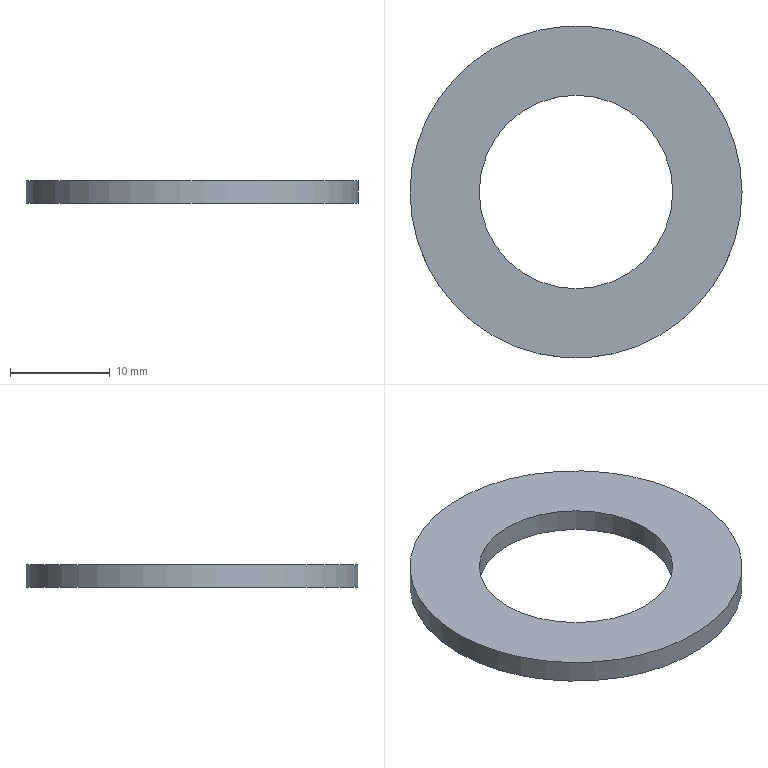Part | NX | features solid 2 | 1 solid | 4 faces | box 33.325 x 33.325 x 2.286 mm | volume 1316 mm3 | cylinder 2 | plane 2 | commonest cylinder face diameters 19.431 x1 33.325 x1
STEP:
#1=CARTESIAN_POINT('',(16.662,0.,2.286));
#2=VERTEX_POINT('',#1);
#3=CARTESIAN_POINT('',(0.,0.,2.286));
#4=DIRECTION('',(0.,0.,-1.));
#5=DIRECTION('',(1.,0.,0.));
#6=AXIS2_PLACEMENT_3D('',#3,#4,#5);
#7=CIRCLE('',#6,16.662);
#8=EDGE_CURVE('',#2,#2,#7,.T.);
#9=ORIENTED_EDGE('',*,*,#8,.T.);
#10=EDGE_LOOP('',(#9));
#11=FACE_BOUND('',#10,.T.);
#12=CARTESIAN_POINT('',(16.662,0.,0.));
#13=VERTEX_POINT('',#12);
#14=CARTESIAN_POINT('',(0.,0.,0.));
#15=DIRECTION('',(0.,0.,-1.));
#16=DIRECTION('',(1.,0.,0.));
#17=AXIS2_PLACEMENT_3D('',#14,#15,#16);
#18=CIRCLE('',#17,16.662);
#19=EDGE_CURVE('',#13,#13,#18,.T.);
#20=ORIENTED_EDGE('',*,*,#19,.F.);
#21=EDGE_LOOP('',(#20));
#22=FACE_BOUND('',#21,.T.);
#23=CARTESIAN_POINT('',(0.,0.,2.286));
#24=DIRECTION('',(0.,0.,-1.));
#25=DIRECTION('',(-1.,0.,0.));
#26=AXIS2_PLACEMENT_3D('',#23,#24,#25);
#27=CYLINDRICAL_SURFACE('',#26,16.662);
#28=ADVANCED_FACE('',(#11,#22),#27,.T.);
#29=CARTESIAN_POINT('',(9.716,0.,2.286));
#30=VERTEX_POINT('',#29);
#31=CARTESIAN_POINT('',(0.,0.,2.286));
#32=DIRECTION('',(0.,0.,-1.));
#33=DIRECTION('',(1.,0.,0.));
#34=AXIS2_PLACEMENT_3D('',#31,#32,#33);
#35=CIRCLE('',#34,9.716);
#36=EDGE_CURVE('',#30,#30,#35,.T.);
#37=ORIENTED_EDGE('',*,*,#36,.F.);
#38=EDGE_LOOP('',(#37));
#39=FACE_BOUND('',#38,.T.);
#40=CARTESIAN_POINT('',(9.716,0.,0.));
#41=VERTEX_POINT('',#40);
#42=CARTESIAN_POINT('',(0.,0.,0.));
#43=DIRECTION('',(0.,0.,-1.));
#44=DIRECTION('',(1.,0.,0.));
#45=AXIS2_PLACEMENT_3D('',#42,#43,#44);
#46=CIRCLE('',#45,9.716);
#47=EDGE_CURVE('',#41,#41,#46,.T.);
#48=ORIENTED_EDGE('',*,*,#47,.T.);
#49=EDGE_LOOP('',(#48));
#50=FACE_BOUND('',#49,.T.);
#51=CARTESIAN_POINT('',(0.,0.,2.286));
#52=DIRECTION('',(0.,0.,-1.));
#53=DIRECTION('',(-1.,0.,0.));
#54=AXIS2_PLACEMENT_3D('',#51,#52,#53);
#55=CYLINDRICAL_SURFACE('',#54,9.716);
#56=ADVANCED_FACE('',(#39,#50),#55,.F.);
#57=ORIENTED_EDGE('',*,*,#8,.F.);
#58=EDGE_LOOP('',(#57));
#59=FACE_BOUND('',#58,.T.);
#60=ORIENTED_EDGE('',*,*,#36,.T.);
#61=EDGE_LOOP('',(#60));
#62=FACE_BOUND('',#61,.T.);
#63=CARTESIAN_POINT('',(0.,0.,2.286));
#64=DIRECTION('',(0.,0.,-1.));
#65=DIRECTION('',(-1.,0.,0.));
#66=AXIS2_PLACEMENT_3D('',#63,#64,#65);
#67=PLANE('',#66);
#68=ADVANCED_FACE('',(#59,#62),#67,.F.);
#69=ORIENTED_EDGE('',*,*,#19,.T.);
#70=EDGE_LOOP('',(#69));
#71=FACE_BOUND('',#70,.T.);
#72=ORIENTED_EDGE('',*,*,#47,.F.);
#73=EDGE_LOOP('',(#72));
#74=FACE_BOUND('',#73,.T.);
#75=CARTESIAN_POINT('',(0.,0.,0.));
#76=DIRECTION('',(0.,0.,-1.));
#77=DIRECTION('',(-1.,0.,0.));
#78=AXIS2_PLACEMENT_3D('',#75,#76,#77);
#79=PLANE('',#78);
#80=ADVANCED_FACE('',(#71,#74),#79,.T.);
#81=CLOSED_SHELL('',(#28,#56,#68,#80));
#82=MANIFOLD_SOLID_BREP('',#81);
#83=(LENGTH_UNIT()NAMED_UNIT(*)SI_UNIT(.MILLI.,.METRE.));
#84=UNCERTAINTY_MEASURE_WITH_UNIT(LENGTH_MEASURE(0.00001),#83,'','');
#85=(NAMED_UNIT(*)PLANE_ANGLE_UNIT()SI_UNIT($,.RADIAN.));
#86=(NAMED_UNIT(*)SI_UNIT($,.STERADIAN.)SOLID_ANGLE_UNIT());
#87=(GEOMETRIC_REPRESENTATION_CONTEXT(3)GLOBAL_UNCERTAINTY_ASSIGNED_CONTEXT((#84))GLOBAL_UNIT_ASSIGNED_CONTEXT((#83,#85,#86))REPRESENTATION_CONTEXT('',''));
#88=ADVANCED_BREP_SHAPE_REPRESENTATION('',(#82),#87);